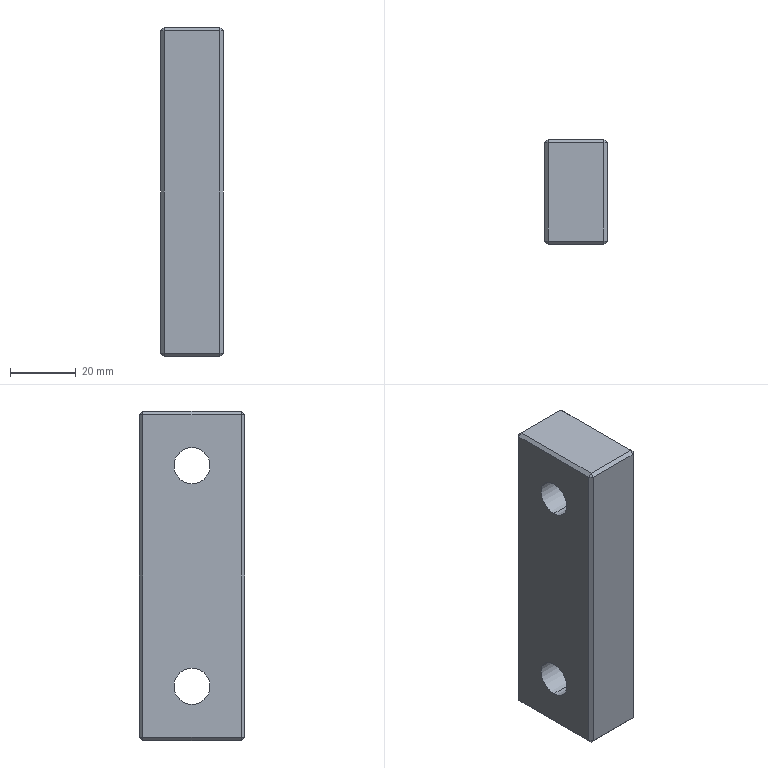Part | SolidWorks | features BaseBody 1 | 1 solid | 36 faces | box 19 x 32 x 100 mm | volume 53384 mm3 | plane 28 | cylinder 8 | commonest cylinder face diameters 11 x4 18 x4
STEP:
#1=CARTESIAN_POINT('',(444.,255.,-24.5));
#2=VERTEX_POINT('',#1);
#3=CARTESIAN_POINT('',(444.,255.,-42.5));
#4=VERTEX_POINT('',#3);
#5=CARTESIAN_POINT('',(444.,255.,-33.5));
#6=DIRECTION('',(1.,0.,0.));
#7=DIRECTION('',(0.,0.,1.));
#8=AXIS2_PLACEMENT_3D('',#5,#6,#7);
#9=CIRCLE('',#8,9.);
#10=EDGE_CURVE('',#2,#4,#9,.T.);
#11=ORIENTED_EDGE('',*,*,#10,.T.);
#12=CARTESIAN_POINT('',(433.,255.,-42.5));
#13=VERTEX_POINT('',#12);
#14=CARTESIAN_POINT('',(444.,255.,-42.5));
#15=DIRECTION('',(-1.,0.,0.));
#16=VECTOR('',#15,1000.);
#17=LINE('',#14,#16);
#18=EDGE_CURVE('',#4,#13,#17,.T.);
#19=ORIENTED_EDGE('',*,*,#18,.T.);
#20=CARTESIAN_POINT('',(433.,255.,-24.5));
#21=VERTEX_POINT('',#20);
#22=CARTESIAN_POINT('',(433.,255.,-33.5));
#23=DIRECTION('',(1.,0.,0.));
#24=DIRECTION('',(0.,0.,1.));
#25=AXIS2_PLACEMENT_3D('',#22,#23,#24);
#26=CIRCLE('',#25,9.);
#27=EDGE_CURVE('',#21,#13,#26,.T.);
#28=ORIENTED_EDGE('',*,*,#27,.F.);
#29=CARTESIAN_POINT('',(444.,255.,-24.5));
#30=DIRECTION('',(-1.,0.,0.));
#31=VECTOR('',#30,1000.);
#32=LINE('',#29,#31);
#33=EDGE_CURVE('',#2,#21,#32,.T.);
#34=ORIENTED_EDGE('',*,*,#33,.F.);
#35=EDGE_LOOP('',(#11,#19,#28,#34));
#36=FACE_OUTER_BOUND('',#35,.T.);
#37=CARTESIAN_POINT('',(444.,255.,-33.5));
#38=DIRECTION('',(-1.,0.,0.));
#39=DIRECTION('',(0.,0.,1.));
#40=AXIS2_PLACEMENT_3D('',#37,#38,#39);
#41=CYLINDRICAL_SURFACE('',#40,9.);
#42=ADVANCED_FACE('',(#36),#41,.F.);
#43=CARTESIAN_POINT('',(433.,255.,-39.));
#44=VERTEX_POINT('',#43);
#45=CARTESIAN_POINT('',(433.,255.,-28.));
#46=VERTEX_POINT('',#45);
#47=CARTESIAN_POINT('',(433.,255.,-33.5));
#48=DIRECTION('',(1.,0.,0.));
#49=DIRECTION('',(0.,0.,1.));
#50=AXIS2_PLACEMENT_3D('',#47,#48,#49);
#51=CIRCLE('',#50,5.5);
#52=EDGE_CURVE('',#44,#46,#51,.T.);
#53=ORIENTED_EDGE('',*,*,#52,.T.);
#54=CARTESIAN_POINT('',(425.,255.,-28.));
#55=VERTEX_POINT('',#54);
#56=CARTESIAN_POINT('',(-56.,255.,-28.));
#57=DIRECTION('',(-1.,0.,0.));
#58=VECTOR('',#57,1000.);
#59=LINE('',#56,#58);
#60=EDGE_CURVE('',#46,#55,#59,.T.);
#61=ORIENTED_EDGE('',*,*,#60,.T.);
#62=CARTESIAN_POINT('',(425.,255.,-39.));
#63=VERTEX_POINT('',#62);
#64=CARTESIAN_POINT('',(425.,255.,-33.5));
#65=DIRECTION('',(1.,0.,0.));
#66=DIRECTION('',(0.,0.,1.));
#67=AXIS2_PLACEMENT_3D('',#64,#65,#66);
#68=CIRCLE('',#67,5.5);
#69=EDGE_CURVE('',#63,#55,#68,.T.);
#70=ORIENTED_EDGE('',*,*,#69,.F.);
#71=CARTESIAN_POINT('',(-56.,255.,-39.));
#72=DIRECTION('',(-1.,0.,0.));
#73=VECTOR('',#72,1000.);
#74=LINE('',#71,#73);
#75=EDGE_CURVE('',#44,#63,#74,.T.);
#76=ORIENTED_EDGE('',*,*,#75,.F.);
#77=EDGE_LOOP('',(#53,#61,#70,#76));
#78=FACE_OUTER_BOUND('',#77,.T.);
#79=CARTESIAN_POINT('',(-56.,255.,-33.5));
#80=DIRECTION('',(-1.,0.,0.));
#81=DIRECTION('',(0.,0.,-1.));
#82=AXIS2_PLACEMENT_3D('',#79,#80,#81);
#83=CYLINDRICAL_SURFACE('',#82,5.5);
#84=ADVANCED_FACE('',(#78),#83,.F.);
#85=CARTESIAN_POINT('',(444.,255.,42.5));
#86=VERTEX_POINT('',#85);
#87=CARTESIAN_POINT('',(444.,255.,24.5));
#88=VERTEX_POINT('',#87);
#89=CARTESIAN_POINT('',(444.,255.,33.5));
#90=DIRECTION('',(1.,0.,0.));
#91=DIRECTION('',(0.,0.,1.));
#92=AXIS2_PLACEMENT_3D('',#89,#90,#91);
#93=CIRCLE('',#92,9.);
#94=EDGE_CURVE('',#86,#88,#93,.T.);
#95=ORIENTED_EDGE('',*,*,#94,.T.);
#96=CARTESIAN_POINT('',(433.,255.,24.5));
#97=VERTEX_POINT('',#96);
#98=CARTESIAN_POINT('',(444.,255.,24.5));
#99=DIRECTION('',(-1.,0.,0.));
#100=VECTOR('',#99,1000.);
#101=LINE('',#98,#100);
#102=EDGE_CURVE('',#88,#97,#101,.T.);
#103=ORIENTED_EDGE('',*,*,#102,.T.);
#104=CARTESIAN_POINT('',(433.,255.,42.5));
#105=VERTEX_POINT('',#104);
#106=CARTESIAN_POINT('',(433.,255.,33.5));
#107=DIRECTION('',(1.,0.,0.));
#108=DIRECTION('',(0.,0.,1.));
#109=AXIS2_PLACEMENT_3D('',#106,#107,#108);
#110=CIRCLE('',#109,9.);
#111=EDGE_CURVE('',#105,#97,#110,.T.);
#112=ORIENTED_EDGE('',*,*,#111,.F.);
#113=CARTESIAN_POINT('',(444.,255.,42.5));
#114=DIRECTION('',(-1.,0.,0.));
#115=VECTOR('',#114,1000.);
#116=LINE('',#113,#115);
#117=EDGE_CURVE('',#86,#105,#116,.T.);
#118=ORIENTED_EDGE('',*,*,#117,.F.);
#119=EDGE_LOOP('',(#95,#103,#112,#118));
#120=FACE_OUTER_BOUND('',#119,.T.);
#121=CARTESIAN_POINT('',(444.,255.,33.5));
#122=DIRECTION('',(-1.,0.,0.));
#123=DIRECTION('',(0.,0.,1.));
#124=AXIS2_PLACEMENT_3D('',#121,#122,#123);
#125=CYLINDRICAL_SURFACE('',#124,9.);
#126=ADVANCED_FACE('',(#120),#125,.F.);
#127=CARTESIAN_POINT('',(433.,255.,28.));
#128=VERTEX_POINT('',#127);
#129=CARTESIAN_POINT('',(433.,255.,39.));
#130=VERTEX_POINT('',#129);
#131=CARTESIAN_POINT('',(433.,255.,33.5));
#132=DIRECTION('',(1.,0.,0.));
#133=DIRECTION('',(0.,0.,1.));
#134=AXIS2_PLACEMENT_3D('',#131,#132,#133);
#135=CIRCLE('',#134,5.5);
#136=EDGE_CURVE('',#128,#130,#135,.T.);
#137=ORIENTED_EDGE('',*,*,#136,.T.);
#138=CARTESIAN_POINT('',(425.,255.,39.));
#139=VERTEX_POINT('',#138);
#140=CARTESIAN_POINT('',(-56.,255.,39.));
#141=DIRECTION('',(-1.,0.,0.));
#142=VECTOR('',#141,1000.);
#143=LINE('',#140,#142);
#144=EDGE_CURVE('',#130,#139,#143,.T.);
#145=ORIENTED_EDGE('',*,*,#144,.T.);
#146=CARTESIAN_POINT('',(425.,255.,28.));
#147=VERTEX_POINT('',#146);
#148=CARTESIAN_POINT('',(425.,255.,33.5));
#149=DIRECTION('',(1.,0.,0.));
#150=DIRECTION('',(0.,0.,1.));
#151=AXIS2_PLACEMENT_3D('',#148,#149,#150);
#152=CIRCLE('',#151,5.5);
#153=EDGE_CURVE('',#147,#139,#152,.T.);
#154=ORIENTED_EDGE('',*,*,#153,.F.);
#155=CARTESIAN_POINT('',(-56.,255.,28.));
#156=DIRECTION('',(-1.,0.,0.));
#157=VECTOR('',#156,1000.);
#158=LINE('',#155,#157);
#159=EDGE_CURVE('',#128,#147,#158,.T.);
#160=ORIENTED_EDGE('',*,*,#159,.F.);
#161=EDGE_LOOP('',(#137,#145,#154,#160));
#162=FACE_OUTER_BOUND('',#161,.T.);
#163=CARTESIAN_POINT('',(-56.,255.,33.5));
#164=DIRECTION('',(-1.,0.,0.));
#165=DIRECTION('',(0.,0.,-1.));
#166=AXIS2_PLACEMENT_3D('',#163,#164,#165);
#167=CYLINDRICAL_SURFACE('',#166,5.5);
#168=ADVANCED_FACE('',(#162),#167,.F.);
#169=CARTESIAN_POINT('',(426.,271.,49.));
#170=VERTEX_POINT('',#169);
#171=CARTESIAN_POINT('',(426.,271.,-49.));
#172=VERTEX_POINT('',#171);
#173=CARTESIAN_POINT('',(426.,271.,-60.));
#174=DIRECTION('',(0.,0.,-1.));
#175=VECTOR('',#174,1000.);
#176=LINE('',#173,#175);
#177=EDGE_CURVE('',#170,#172,#176,.T.);
#178=ORIENTED_EDGE('',*,*,#177,.F.);
#179=CARTESIAN_POINT('',(443.,271.,49.));
#180=VERTEX_POINT('',#179);
#181=CARTESIAN_POINT('',(434.5,271.,49.));
#182=DIRECTION('',(-1.,0.,0.));
#183=VECTOR('',#182,1000.);
#184=LINE('',#181,#183);
#185=EDGE_CURVE('',#180,#170,#184,.T.);
#186=ORIENTED_EDGE('',*,*,#185,.F.);
#187=CARTESIAN_POINT('',(443.,271.,-49.));
#188=VERTEX_POINT('',#187);
#189=CARTESIAN_POINT('',(443.,271.,-60.));
#190=DIRECTION('',(0.,0.,1.));
#191=VECTOR('',#190,1000.);
#192=LINE('',#189,#191);
#193=EDGE_CURVE('',#188,#180,#192,.T.);
#194=ORIENTED_EDGE('',*,*,#193,.F.);
#195=CARTESIAN_POINT('',(444.,271.,-49.));
#196=DIRECTION('',(1.,0.,0.));
#197=VECTOR('',#196,1000.);
#198=LINE('',#195,#197);
#199=EDGE_CURVE('',#172,#188,#198,.T.);
#200=ORIENTED_EDGE('',*,*,#199,.F.);
#201=EDGE_LOOP('',(#178,#186,#194,#200));
#202=FACE_OUTER_BOUND('',#201,.T.);
#203=CARTESIAN_POINT('',(434.5,271.,-60.));
#204=DIRECTION('',(0.,1.,0.));
#205=DIRECTION('',(0.,0.,-1.));
#206=AXIS2_PLACEMENT_3D('',#203,#204,#205);
#207=PLANE('',#206);
#208=ADVANCED_FACE('',(#202),#207,.T.);
#209=CARTESIAN_POINT('',(426.,270.,-50.));
#210=VERTEX_POINT('',#209);
#211=CARTESIAN_POINT('',(426.,240.,-50.));
#212=VERTEX_POINT('',#211);
#213=CARTESIAN_POINT('',(426.,239.,-50.));
#214=DIRECTION('',(0.,-1.,0.));
#215=VECTOR('',#214,1000.);
#216=LINE('',#213,#215);
#217=EDGE_CURVE('',#210,#212,#216,.T.);
#218=ORIENTED_EDGE('',*,*,#217,.F.);
#219=CARTESIAN_POINT('',(443.,270.,-50.));
#220=VERTEX_POINT('',#219);
#221=CARTESIAN_POINT('',(425.,270.,-50.));
#222=DIRECTION('',(-1.,0.,0.));
#223=VECTOR('',#222,1000.);
#224=LINE('',#221,#223);
#225=EDGE_CURVE('',#220,#210,#224,.T.);
#226=ORIENTED_EDGE('',*,*,#225,.F.);
#227=CARTESIAN_POINT('',(443.,240.,-50.));
#228=VERTEX_POINT('',#227);
#229=CARTESIAN_POINT('',(443.,271.,-50.));
#230=DIRECTION('',(0.,1.,0.));
#231=VECTOR('',#230,1000.);
#232=LINE('',#229,#231);
#233=EDGE_CURVE('',#228,#220,#232,.T.);
#234=ORIENTED_EDGE('',*,*,#233,.F.);
#235=CARTESIAN_POINT('',(135.,240.,-50.));
#236=DIRECTION('',(1.,0.,0.));
#237=VECTOR('',#236,1000.);
#238=LINE('',#235,#237);
#239=EDGE_CURVE('',#212,#228,#238,.T.);
#240=ORIENTED_EDGE('',*,*,#239,.F.);
#241=EDGE_LOOP('',(#218,#226,#234,#240));
#242=FACE_OUTER_BOUND('',#241,.T.);
#243=CARTESIAN_POINT('',(135.,111.,-50.));
#244=DIRECTION('',(0.,0.,1.));
#245=DIRECTION('',(1.,0.,0.));
#246=AXIS2_PLACEMENT_3D('',#243,#244,#245);
#247=PLANE('',#246);
#248=ADVANCED_FACE('',(#242),#247,.F.);
#249=ORIENTED_EDGE('',*,*,#10,.F.);
#250=CARTESIAN_POINT('',(444.,255.,-33.5));
#251=DIRECTION('',(1.,0.,0.));
#252=DIRECTION('',(0.,0.,1.));
#253=AXIS2_PLACEMENT_3D('',#250,#251,#252);
#254=CIRCLE('',#253,9.);
#255=EDGE_CURVE('',#4,#2,#254,.T.);
#256=ORIENTED_EDGE('',*,*,#255,.F.);
#257=EDGE_LOOP('',(#249,#256));
#258=FACE_BOUND('',#257,.T.);
#259=ORIENTED_EDGE('',*,*,#94,.F.);
#260=CARTESIAN_POINT('',(444.,255.,33.5));
#261=DIRECTION('',(1.,0.,0.));
#262=DIRECTION('',(0.,0.,1.));
#263=AXIS2_PLACEMENT_3D('',#260,#261,#262);
#264=CIRCLE('',#263,9.);
#265=EDGE_CURVE('',#88,#86,#264,.T.);
#266=ORIENTED_EDGE('',*,*,#265,.F.);
#267=EDGE_LOOP('',(#259,#266));
#268=FACE_BOUND('',#267,.T.);
#269=CARTESIAN_POINT('',(444.,270.,49.));
#270=VERTEX_POINT('',#269);
#271=CARTESIAN_POINT('',(444.,270.,-49.));
#272=VERTEX_POINT('',#271);
#273=CARTESIAN_POINT('',(444.,270.,-60.));
#274=DIRECTION('',(0.,0.,-1.));
#275=VECTOR('',#274,1000.);
#276=LINE('',#273,#275);
#277=EDGE_CURVE('',#270,#272,#276,.T.);
#278=ORIENTED_EDGE('',*,*,#277,.F.);
#279=CARTESIAN_POINT('',(444.,240.,49.));
#280=VERTEX_POINT('',#279);
#281=CARTESIAN_POINT('',(444.,251.,49.));
#282=DIRECTION('',(0.,1.,0.));
#283=VECTOR('',#282,1000.);
#284=LINE('',#281,#283);
#285=EDGE_CURVE('',#280,#270,#284,.T.);
#286=ORIENTED_EDGE('',*,*,#285,.F.);
#287=CARTESIAN_POINT('',(444.,240.,-49.));
#288=VERTEX_POINT('',#287);
#289=CARTESIAN_POINT('',(444.,240.,50.));
#290=DIRECTION('',(0.,0.,1.));
#291=VECTOR('',#290,1000.);
#292=LINE('',#289,#291);
#293=EDGE_CURVE('',#288,#280,#292,.T.);
#294=ORIENTED_EDGE('',*,*,#293,.F.);
#295=CARTESIAN_POINT('',(444.,239.,-49.));
#296=DIRECTION('',(0.,-1.,0.));
#297=VECTOR('',#296,1000.);
#298=LINE('',#295,#297);
#299=EDGE_CURVE('',#272,#288,#298,.T.);
#300=ORIENTED_EDGE('',*,*,#299,.F.);
#301=EDGE_LOOP('',(#278,#286,#294,#300));
#302=FACE_OUTER_BOUND('',#301,.T.);
#303=CARTESIAN_POINT('',(444.,251.,-60.));
#304=DIRECTION('',(1.,0.,0.));
#305=DIRECTION('',(0.,0.,-1.));
#306=AXIS2_PLACEMENT_3D('',#303,#304,#305);
#307=PLANE('',#306);
#308=ADVANCED_FACE('',(#258,#268,#302),#307,.T.);
#309=ORIENTED_EDGE('',*,*,#69,.T.);
#310=CARTESIAN_POINT('',(425.,255.,-33.5));
#311=DIRECTION('',(1.,0.,0.));
#312=DIRECTION('',(0.,0.,1.));
#313=AXIS2_PLACEMENT_3D('',#310,#311,#312);
#314=CIRCLE('',#313,5.5);
#315=EDGE_CURVE('',#55,#63,#314,.T.);
#316=ORIENTED_EDGE('',*,*,#315,.T.);
#317=EDGE_LOOP('',(#309,#316));
#318=FACE_BOUND('',#317,.T.);
#319=ORIENTED_EDGE('',*,*,#153,.T.);
#320=CARTESIAN_POINT('',(425.,255.,33.5));
#321=DIRECTION('',(1.,0.,0.));
#322=DIRECTION('',(0.,0.,1.));
#323=AXIS2_PLACEMENT_3D('',#320,#321,#322);
#324=CIRCLE('',#323,5.5);
#325=EDGE_CURVE('',#139,#147,#324,.T.);
#326=ORIENTED_EDGE('',*,*,#325,.T.);
#327=EDGE_LOOP('',(#319,#326));
#328=FACE_BOUND('',#327,.T.);
#329=CARTESIAN_POINT('',(425.,240.,-49.));
#330=VERTEX_POINT('',#329);
#331=CARTESIAN_POINT('',(425.,270.,-49.));
#332=VERTEX_POINT('',#331);
#333=CARTESIAN_POINT('',(425.,271.,-49.));
#334=DIRECTION('',(0.,1.,0.));
#335=VECTOR('',#334,1000.);
#336=LINE('',#333,#335);
#337=EDGE_CURVE('',#330,#332,#336,.T.);
#338=ORIENTED_EDGE('',*,*,#337,.F.);
#339=CARTESIAN_POINT('',(425.,240.,49.));
#340=VERTEX_POINT('',#339);
#341=CARTESIAN_POINT('',(425.,240.,-50.));
#342=DIRECTION('',(0.,0.,-1.));
#343=VECTOR('',#342,1000.);
#344=LINE('',#341,#343);
#345=EDGE_CURVE('',#340,#330,#344,.T.);
#346=ORIENTED_EDGE('',*,*,#345,.F.);
#347=CARTESIAN_POINT('',(425.,270.,49.));
#348=VERTEX_POINT('',#347);
#349=CARTESIAN_POINT('',(425.,251.,49.));
#350=DIRECTION('',(0.,-1.,0.));
#351=VECTOR('',#350,1000.);
#352=LINE('',#349,#351);
#353=EDGE_CURVE('',#348,#340,#352,.T.);
#354=ORIENTED_EDGE('',*,*,#353,.F.);
#355=CARTESIAN_POINT('',(425.,270.,-60.));
#356=DIRECTION('',(0.,0.,1.));
#357=VECTOR('',#356,1000.);
#358=LINE('',#355,#357);
#359=EDGE_CURVE('',#332,#348,#358,.T.);
#360=ORIENTED_EDGE('',*,*,#359,.F.);
#361=EDGE_LOOP('',(#338,#346,#354,#360));
#362=FACE_OUTER_BOUND('',#361,.T.);
#363=CARTESIAN_POINT('',(425.,251.,-60.));
#364=DIRECTION('',(-1.,0.,0.));
#365=DIRECTION('',(0.,0.,1.));
#366=AXIS2_PLACEMENT_3D('',#363,#364,#365);
#367=PLANE('',#366);
#368=ADVANCED_FACE('',(#318,#328,#362),#367,.T.);
#369=CARTESIAN_POINT('',(443.,270.,50.));
#370=VERTEX_POINT('',#369);
#371=CARTESIAN_POINT('',(443.,240.,50.));
#372=VERTEX_POINT('',#371);
#373=CARTESIAN_POINT('',(443.,251.,50.));
#374=DIRECTION('',(0.,-1.,0.));
#375=VECTOR('',#374,1000.);
#376=LINE('',#373,#375);
#377=EDGE_CURVE('',#370,#372,#376,.T.);
#378=ORIENTED_EDGE('',*,*,#377,.F.);
#379=CARTESIAN_POINT('',(426.,270.,50.));
#380=VERTEX_POINT('',#379);
#381=CARTESIAN_POINT('',(434.5,270.,50.));
#382=DIRECTION('',(1.,0.,0.));
#383=VECTOR('',#382,1000.);
#384=LINE('',#381,#383);
#385=EDGE_CURVE('',#380,#370,#384,.T.);
#386=ORIENTED_EDGE('',*,*,#385,.F.);
#387=CARTESIAN_POINT('',(426.,240.,50.));
#388=VERTEX_POINT('',#387);
#389=CARTESIAN_POINT('',(426.,251.,50.));
#390=DIRECTION('',(0.,1.,0.));
#391=VECTOR('',#390,1000.);
#392=LINE('',#389,#391);
#393=EDGE_CURVE('',#388,#380,#392,.T.);
#394=ORIENTED_EDGE('',*,*,#393,.F.);
#395=CARTESIAN_POINT('',(425.,240.,50.));
#396=DIRECTION('',(-1.,0.,0.));
#397=VECTOR('',#396,1000.);
#398=LINE('',#395,#397);
#399=EDGE_CURVE('',#372,#388,#398,.T.);
#400=ORIENTED_EDGE('',*,*,#399,.F.);
#401=EDGE_LOOP('',(#378,#386,#394,#400));
#402=FACE_OUTER_BOUND('',#401,.T.);
#403=CARTESIAN_POINT('',(434.5,251.,50.));
#404=DIRECTION('',(0.,0.,1.));
#405=DIRECTION('',(1.,0.,0.));
#406=AXIS2_PLACEMENT_3D('',#403,#404,#405);
#407=PLANE('',#406);
#408=ADVANCED_FACE('',(#402),#407,.T.);
#409=CARTESIAN_POINT('',(443.,239.,49.));
#410=VERTEX_POINT('',#409);
#411=CARTESIAN_POINT('',(443.,239.,-49.));
#412=VERTEX_POINT('',#411);
#413=CARTESIAN_POINT('',(443.,239.,-50.));
#414=DIRECTION('',(0.,0.,-1.));
#415=VECTOR('',#414,1000.);
#416=LINE('',#413,#415);
#417=EDGE_CURVE('',#410,#412,#416,.T.);
#418=ORIENTED_EDGE('',*,*,#417,.F.);
#419=CARTESIAN_POINT('',(426.,239.,49.));
#420=VERTEX_POINT('',#419);
#421=CARTESIAN_POINT('',(444.,239.,49.));
#422=DIRECTION('',(1.,0.,0.));
#423=VECTOR('',#422,1000.);
#424=LINE('',#421,#423);
#425=EDGE_CURVE('',#420,#410,#424,.T.);
#426=ORIENTED_EDGE('',*,*,#425,.F.);
#427=CARTESIAN_POINT('',(426.,239.,-49.));
#428=VERTEX_POINT('',#427);
#429=CARTESIAN_POINT('',(426.,239.,50.));
#430=DIRECTION('',(0.,0.,1.));
#431=VECTOR('',#430,1000.);
#432=LINE('',#429,#431);
#433=EDGE_CURVE('',#428,#420,#432,.T.);
#434=ORIENTED_EDGE('',*,*,#433,.F.);
#435=CARTESIAN_POINT('',(434.5,239.,-49.));
#436=DIRECTION('',(-1.,0.,0.));
#437=VECTOR('',#436,1000.);
#438=LINE('',#435,#437);
#439=EDGE_CURVE('',#412,#428,#438,.T.);
#440=ORIENTED_EDGE('',*,*,#439,.F.);
#441=EDGE_LOOP('',(#418,#426,#434,#440));
#442=FACE_OUTER_BOUND('',#441,.T.);
#443=CARTESIAN_POINT('',(434.5,239.,0.));
#444=DIRECTION('',(0.,1.,0.));
#445=DIRECTION('',(0.,0.,-1.));
#446=AXIS2_PLACEMENT_3D('',#443,#444,#445);
#447=PLANE('',#446);
#448=ADVANCED_FACE('',(#442),#447,.F.);
#449=CARTESIAN_POINT('',(426.,270.5,49.5));
#450=DIRECTION('',(0.,-0.7071,0.7071));
#451=VECTOR('',#450,1000.);
#452=LINE('',#449,#451);
#453=EDGE_CURVE('',#170,#380,#452,.T.);
#454=ORIENTED_EDGE('',*,*,#453,.T.);
#455=ORIENTED_EDGE('',*,*,#385,.T.);
#456=CARTESIAN_POINT('',(443.,271.,49.));
#457=DIRECTION('',(0.,0.7071,-0.7071));
#458=VECTOR('',#457,1000.);
#459=LINE('',#456,#458);
#460=EDGE_CURVE('',#370,#180,#459,.T.);
#461=ORIENTED_EDGE('',*,*,#460,.T.);
#462=ORIENTED_EDGE('',*,*,#185,.T.);
#463=EDGE_LOOP('',(#454,#455,#461,#462));
#464=FACE_OUTER_BOUND('',#463,.T.);
#465=CARTESIAN_POINT('',(434.5,271.,49.));
#466=DIRECTION('',(0.,-0.7071,-0.7071));
#467=DIRECTION('',(0.,-0.7071,0.7071));
#468=AXIS2_PLACEMENT_3D('',#465,#466,#467);
#469=PLANE('',#468);
#470=ADVANCED_FACE('',(#464),#469,.F.);
#471=CARTESIAN_POINT('',(425.,270.,49.));
#472=DIRECTION('',(-0.7071,-0.7071,0.));
#473=VECTOR('',#472,1000.);
#474=LINE('',#471,#473);
#475=EDGE_CURVE('',#170,#348,#474,.T.);
#476=ORIENTED_EDGE('',*,*,#475,.T.);
#477=CARTESIAN_POINT('',(425.,270.,49.));
#478=DIRECTION('',(0.7071,0.,0.7071));
#479=VECTOR('',#478,1000.);
#480=LINE('',#477,#479);
#481=EDGE_CURVE('',#348,#380,#480,.T.);
#482=ORIENTED_EDGE('',*,*,#481,.T.);
#483=ORIENTED_EDGE('',*,*,#453,.F.);
#484=EDGE_LOOP('',(#476,#482,#483));
#485=FACE_OUTER_BOUND('',#484,.T.);
#486=CARTESIAN_POINT('',(425.,270.,49.));
#487=DIRECTION('',(-0.5774,0.5774,0.5774));
#488=DIRECTION('',(0.7071,0.,0.7071));
#489=AXIS2_PLACEMENT_3D('',#486,#487,#488);
#490=PLANE('',#489);
#491=ADVANCED_FACE('',(#485),#490,.T.);
#492=CARTESIAN_POINT('',(443.5,270.,49.5));
#493=DIRECTION('',(0.7071,0.,-0.7071));
#494=VECTOR('',#493,1000.);
#495=LINE('',#492,#494);
#496=EDGE_CURVE('',#370,#270,#495,.T.);
#497=ORIENTED_EDGE('',*,*,#496,.T.);
#498=CARTESIAN_POINT('',(443.,271.,49.));
#499=DIRECTION('',(-0.7071,0.7071,0.));
#500=VECTOR('',#499,1000.);
#501=LINE('',#498,#500);
#502=EDGE_CURVE('',#270,#180,#501,.T.);
#503=ORIENTED_EDGE('',*,*,#502,.T.);
#504=ORIENTED_EDGE('',*,*,#460,.F.);
#505=EDGE_LOOP('',(#497,#503,#504));
#506=FACE_OUTER_BOUND('',#505,.T.);
#507=CARTESIAN_POINT('',(443.,271.,49.));
#508=DIRECTION('',(0.5774,0.5774,0.5774));
#509=DIRECTION('',(0.7071,0.,-0.7071));
#510=AXIS2_PLACEMENT_3D('',#507,#508,#509);
#511=PLANE('',#510);
#512=ADVANCED_FACE('',(#506),#511,.T.);
#513=ORIENTED_EDGE('',*,*,#481,.F.);
#514=ORIENTED_EDGE('',*,*,#353,.T.);
#515=CARTESIAN_POINT('',(426.,240.,50.));
#516=DIRECTION('',(0.7071,0.,0.7071));
#517=VECTOR('',#516,1000.);
#518=LINE('',#515,#517);
#519=EDGE_CURVE('',#340,#388,#518,.T.);
#520=ORIENTED_EDGE('',*,*,#519,.T.);
#521=ORIENTED_EDGE('',*,*,#393,.T.);
#522=EDGE_LOOP('',(#513,#514,#520,#521));
#523=FACE_OUTER_BOUND('',#522,.T.);
#524=CARTESIAN_POINT('',(425.,251.,49.));
#525=DIRECTION('',(0.7071,0.,-0.7071));
#526=DIRECTION('',(-0.7071,0.,-0.7071));
#527=AXIS2_PLACEMENT_3D('',#524,#525,#526);
#528=PLANE('',#527);
#529=ADVANCED_FACE('',(#523),#528,.F.);
#530=ORIENTED_EDGE('',*,*,#475,.F.);
#531=ORIENTED_EDGE('',*,*,#177,.T.);
#532=CARTESIAN_POINT('',(426.,271.,-49.));
#533=DIRECTION('',(-0.7071,-0.7071,0.));
#534=VECTOR('',#533,1000.);
#535=LINE('',#532,#534);
#536=EDGE_CURVE('',#172,#332,#535,.T.);
#537=ORIENTED_EDGE('',*,*,#536,.T.);
#538=ORIENTED_EDGE('',*,*,#359,.T.);
#539=EDGE_LOOP('',(#530,#531,#537,#538));
#540=FACE_OUTER_BOUND('',#539,.T.);
#541=CARTESIAN_POINT('',(425.,270.,-60.));
#542=DIRECTION('',(0.7071,-0.7071,0.));
#543=DIRECTION('',(-0.7071,-0.7071,0.));
#544=AXIS2_PLACEMENT_3D('',#541,#542,#543);
#545=PLANE('',#544);
#546=ADVANCED_FACE('',(#540),#545,.F.);
#547=CARTESIAN_POINT('',(443.,270.,-50.));
#548=DIRECTION('',(0.,-0.7071,-0.7071));
#549=VECTOR('',#548,1000.);
#550=LINE('',#547,#549);
#551=EDGE_CURVE('',#188,#220,#550,.T.);
#552=ORIENTED_EDGE('',*,*,#551,.T.);
#553=ORIENTED_EDGE('',*,*,#225,.T.);
#554=CARTESIAN_POINT('',(426.,271.,-49.));
#555=DIRECTION('',(0.,0.7071,0.7071));
#556=VECTOR('',#555,1000.);
#557=LINE('',#554,#556);
#558=EDGE_CURVE('',#210,#172,#557,.T.);
#559=ORIENTED_EDGE('',*,*,#558,.T.);
#560=ORIENTED_EDGE('',*,*,#199,.T.);
#561=EDGE_LOOP('',(#552,#553,#559,#560));
#562=FACE_OUTER_BOUND('',#561,.T.);
#563=CARTESIAN_POINT('',(135.,270.,-50.));
#564=DIRECTION('',(0.,0.7071,-0.7071));
#565=DIRECTION('',(0.,-0.7071,-0.7071));
#566=AXIS2_PLACEMENT_3D('',#563,#564,#565);
#567=PLANE('',#566);
#568=ADVANCED_FACE('',(#562),#567,.T.);
#569=ORIENTED_EDGE('',*,*,#502,.F.);
#570=ORIENTED_EDGE('',*,*,#277,.T.);
#571=CARTESIAN_POINT('',(443.5,270.5,-49.));
#572=DIRECTION('',(-0.7071,0.7071,0.));
#573=VECTOR('',#572,1000.);
#574=LINE('',#571,#573);
#575=EDGE_CURVE('',#272,#188,#574,.T.);
#576=ORIENTED_EDGE('',*,*,#575,.T.);
#577=ORIENTED_EDGE('',*,*,#193,.T.);
#578=EDGE_LOOP('',(#569,#570,#576,#577));
#579=FACE_OUTER_BOUND('',#578,.T.);
#580=CARTESIAN_POINT('',(443.,271.,-60.));
#581=DIRECTION('',(-0.7071,-0.7071,0.));
#582=DIRECTION('',(-0.7071,0.7071,0.));
#583=AXIS2_PLACEMENT_3D('',#580,#581,#582);
#584=PLANE('',#583);
#585=ADVANCED_FACE('',(#579),#584,.F.);
#586=ORIENTED_EDGE('',*,*,#496,.F.);
#587=ORIENTED_EDGE('',*,*,#377,.T.);
#588=CARTESIAN_POINT('',(444.,240.,49.));
#589=DIRECTION('',(0.7071,0.,-0.7071));
#590=VECTOR('',#589,1000.);
#591=LINE('',#588,#590);
#592=EDGE_CURVE('',#372,#280,#591,.T.);
#593=ORIENTED_EDGE('',*,*,#592,.T.);
#594=ORIENTED_EDGE('',*,*,#285,.T.);
#595=EDGE_LOOP('',(#586,#587,#593,#594));
#596=FACE_OUTER_BOUND('',#595,.T.);
#597=CARTESIAN_POINT('',(444.,251.,49.));
#598=DIRECTION('',(-0.7071,0.,-0.7071));
#599=DIRECTION('',(-0.7071,0.,0.7071));
#600=AXIS2_PLACEMENT_3D('',#597,#598,#599);
#601=PLANE('',#600);
#602=ADVANCED_FACE('',(#596),#601,.F.);
#603=CARTESIAN_POINT('',(426.,240.,50.));
#604=DIRECTION('',(0.,-0.7071,-0.7071));
#605=VECTOR('',#604,1000.);
#606=LINE('',#603,#605);
#607=EDGE_CURVE('',#388,#420,#606,.T.);
#608=ORIENTED_EDGE('',*,*,#607,.T.);
#609=ORIENTED_EDGE('',*,*,#425,.T.);
#610=CARTESIAN_POINT('',(443.,239.5,49.5));
#611=DIRECTION('',(0.,0.7071,0.7071));
#612=VECTOR('',#611,1000.);
#613=LINE('',#610,#612);
#614=EDGE_CURVE('',#410,#372,#613,.T.);
#615=ORIENTED_EDGE('',*,*,#614,.T.);
#616=ORIENTED_EDGE('',*,*,#399,.T.);
#617=EDGE_LOOP('',(#608,#609,#615,#616));
#618=FACE_OUTER_BOUND('',#617,.T.);
#619=CARTESIAN_POINT('',(434.5,239.,49.));
#620=DIRECTION('',(0.,-0.7071,0.7071));
#621=DIRECTION('',(0.,0.7071,0.7071));
#622=AXIS2_PLACEMENT_3D('',#619,#620,#621);
#623=PLANE('',#622);
#624=ADVANCED_FACE('',(#618),#623,.T.);
#625=ORIENTED_EDGE('',*,*,#519,.F.);
#626=CARTESIAN_POINT('',(425.5,239.5,49.));
#627=DIRECTION('',(0.7071,-0.7071,0.));
#628=VECTOR('',#627,1000.);
#629=LINE('',#626,#628);
#630=EDGE_CURVE('',#340,#420,#629,.T.);
#631=ORIENTED_EDGE('',*,*,#630,.T.);
#632=ORIENTED_EDGE('',*,*,#607,.F.);
#633=EDGE_LOOP('',(#625,#631,#632));
#634=FACE_OUTER_BOUND('',#633,.T.);
#635=CARTESIAN_POINT('',(426.,240.,50.));
#636=DIRECTION('',(-0.5774,-0.5774,0.5774));
#637=DIRECTION('',(0.7071,0.,0.7071));
#638=AXIS2_PLACEMENT_3D('',#635,#636,#637);
#639=PLANE('',#638);
#640=ADVANCED_FACE('',(#634),#639,.T.);
#641=ORIENTED_EDGE('',*,*,#558,.F.);
#642=CARTESIAN_POINT('',(425.5,270.,-49.5));
#643=DIRECTION('',(-0.7071,0.,0.7071));
#644=VECTOR('',#643,1000.);
#645=LINE('',#642,#644);
#646=EDGE_CURVE('',#210,#332,#645,.T.);
#647=ORIENTED_EDGE('',*,*,#646,.T.);
#648=ORIENTED_EDGE('',*,*,#536,.F.);
#649=EDGE_LOOP('',(#641,#647,#648));
#650=FACE_OUTER_BOUND('',#649,.T.);
#651=CARTESIAN_POINT('',(426.,271.,-49.));
#652=DIRECTION('',(-0.5774,0.5774,-0.5774));
#653=DIRECTION('',(-0.7071,0.,0.7071));
#654=AXIS2_PLACEMENT_3D('',#651,#652,#653);
#655=PLANE('',#654);
#656=ADVANCED_FACE('',(#650),#655,.T.);
#657=ORIENTED_EDGE('',*,*,#575,.F.);
#658=CARTESIAN_POINT('',(443.,270.,-50.));
#659=DIRECTION('',(-0.7071,0.,-0.7071));
#660=VECTOR('',#659,1000.);
#661=LINE('',#658,#660);
#662=EDGE_CURVE('',#272,#220,#661,.T.);
#663=ORIENTED_EDGE('',*,*,#662,.T.);
#664=ORIENTED_EDGE('',*,*,#551,.F.);
#665=EDGE_LOOP('',(#657,#663,#664));
#666=FACE_OUTER_BOUND('',#665,.T.);
#667=CARTESIAN_POINT('',(443.,270.,-50.));
#668=DIRECTION('',(0.5774,0.5774,-0.5774));
#669=DIRECTION('',(-0.7071,0.,-0.7071));
#670=AXIS2_PLACEMENT_3D('',#667,#668,#669);
#671=PLANE('',#670);
#672=ADVANCED_FACE('',(#666),#671,.T.);
#673=ORIENTED_EDGE('',*,*,#614,.F.);
#674=CARTESIAN_POINT('',(444.,240.,49.));
#675=DIRECTION('',(0.7071,0.7071,0.));
#676=VECTOR('',#675,1000.);
#677=LINE('',#674,#676);
#678=EDGE_CURVE('',#410,#280,#677,.T.);
#679=ORIENTED_EDGE('',*,*,#678,.T.);
#680=ORIENTED_EDGE('',*,*,#592,.F.);
#681=EDGE_LOOP('',(#673,#679,#680));
#682=FACE_OUTER_BOUND('',#681,.T.);
#683=CARTESIAN_POINT('',(444.,240.,49.));
#684=DIRECTION('',(0.5774,-0.5774,0.5774));
#685=DIRECTION('',(0.7071,0.,-0.7071));
#686=AXIS2_PLACEMENT_3D('',#683,#684,#685);
#687=PLANE('',#686);
#688=ADVANCED_FACE('',(#682),#687,.T.);
#689=ORIENTED_EDGE('',*,*,#630,.F.);
#690=ORIENTED_EDGE('',*,*,#345,.T.);
#691=CARTESIAN_POINT('',(426.,239.,-49.));
#692=DIRECTION('',(0.7071,-0.7071,0.));
#693=VECTOR('',#692,1000.);
#694=LINE('',#691,#693);
#695=EDGE_CURVE('',#330,#428,#694,.T.);
#696=ORIENTED_EDGE('',*,*,#695,.T.);
#697=ORIENTED_EDGE('',*,*,#433,.T.);
#698=EDGE_LOOP('',(#689,#690,#696,#697));
#699=FACE_OUTER_BOUND('',#698,.T.);
#700=CARTESIAN_POINT('',(426.,239.,0.));
#701=DIRECTION('',(-0.7071,-0.7071,0.));
#702=DIRECTION('',(-0.7071,0.7071,0.));
#703=AXIS2_PLACEMENT_3D('',#700,#701,#702);
#704=PLANE('',#703);
#705=ADVANCED_FACE('',(#699),#704,.T.);
#706=ORIENTED_EDGE('',*,*,#646,.F.);
#707=ORIENTED_EDGE('',*,*,#217,.T.);
#708=CARTESIAN_POINT('',(425.5,240.,-49.5));
#709=DIRECTION('',(-0.7071,0.,0.7071));
#710=VECTOR('',#709,1000.);
#711=LINE('',#708,#710);
#712=EDGE_CURVE('',#212,#330,#711,.T.);
#713=ORIENTED_EDGE('',*,*,#712,.T.);
#714=ORIENTED_EDGE('',*,*,#337,.T.);
#715=EDGE_LOOP('',(#706,#707,#713,#714));
#716=FACE_OUTER_BOUND('',#715,.T.);
#717=CARTESIAN_POINT('',(426.,111.,-50.));
#718=DIRECTION('',(-0.7071,0.,-0.7071));
#719=DIRECTION('',(-0.7071,0.,0.7071));
#720=AXIS2_PLACEMENT_3D('',#717,#718,#719);
#721=PLANE('',#720);
#722=ADVANCED_FACE('',(#716),#721,.T.);
#723=ORIENTED_EDGE('',*,*,#662,.F.);
#724=ORIENTED_EDGE('',*,*,#299,.T.);
#725=CARTESIAN_POINT('',(443.,240.,-50.));
#726=DIRECTION('',(-0.7071,0.,-0.7071));
#727=VECTOR('',#726,1000.);
#728=LINE('',#725,#727);
#729=EDGE_CURVE('',#288,#228,#728,.T.);
#730=ORIENTED_EDGE('',*,*,#729,.T.);
#731=ORIENTED_EDGE('',*,*,#233,.T.);
#732=EDGE_LOOP('',(#723,#724,#730,#731));
#733=FACE_OUTER_BOUND('',#732,.T.);
#734=CARTESIAN_POINT('',(443.,111.,-50.));
#735=DIRECTION('',(0.7071,0.,-0.7071));
#736=DIRECTION('',(-0.7071,0.,-0.7071));
#737=AXIS2_PLACEMENT_3D('',#734,#735,#736);
#738=PLANE('',#737);
#739=ADVANCED_FACE('',(#733),#738,.T.);
#740=ORIENTED_EDGE('',*,*,#678,.F.);
#741=ORIENTED_EDGE('',*,*,#417,.T.);
#742=CARTESIAN_POINT('',(443.5,239.5,-49.));
#743=DIRECTION('',(0.7071,0.7071,0.));
#744=VECTOR('',#743,1000.);
#745=LINE('',#742,#744);
#746=EDGE_CURVE('',#412,#288,#745,.T.);
#747=ORIENTED_EDGE('',*,*,#746,.T.);
#748=ORIENTED_EDGE('',*,*,#293,.T.);
#749=EDGE_LOOP('',(#740,#741,#747,#748));
#750=FACE_OUTER_BOUND('',#749,.T.);
#751=CARTESIAN_POINT('',(443.,239.,0.));
#752=DIRECTION('',(0.7071,-0.7071,0.));
#753=DIRECTION('',(-0.7071,-0.7071,0.));
#754=AXIS2_PLACEMENT_3D('',#751,#752,#753);
#755=PLANE('',#754);
#756=ADVANCED_FACE('',(#750),#755,.T.);
#757=ORIENTED_EDGE('',*,*,#712,.F.);
#758=CARTESIAN_POINT('',(426.,239.,-49.));
#759=DIRECTION('',(0.,-0.7071,0.7071));
#760=VECTOR('',#759,1000.);
#761=LINE('',#758,#760);
#762=EDGE_CURVE('',#212,#428,#761,.T.);
#763=ORIENTED_EDGE('',*,*,#762,.T.);
#764=ORIENTED_EDGE('',*,*,#695,.F.);
#765=EDGE_LOOP('',(#757,#763,#764));
#766=FACE_OUTER_BOUND('',#765,.T.);
#767=CARTESIAN_POINT('',(426.,239.,-49.));
#768=DIRECTION('',(-0.5774,-0.5774,-0.5774));
#769=DIRECTION('',(-0.7071,0.,0.7071));
#770=AXIS2_PLACEMENT_3D('',#767,#768,#769);
#771=PLANE('',#770);
#772=ADVANCED_FACE('',(#766),#771,.T.);
#773=ORIENTED_EDGE('',*,*,#746,.F.);
#774=CARTESIAN_POINT('',(443.,240.,-50.));
#775=DIRECTION('',(0.,0.7071,-0.7071));
#776=VECTOR('',#775,1000.);
#777=LINE('',#774,#776);
#778=EDGE_CURVE('',#412,#228,#777,.T.);
#779=ORIENTED_EDGE('',*,*,#778,.T.);
#780=ORIENTED_EDGE('',*,*,#729,.F.);
#781=EDGE_LOOP('',(#773,#779,#780));
#782=FACE_OUTER_BOUND('',#781,.T.);
#783=CARTESIAN_POINT('',(443.,240.,-50.));
#784=DIRECTION('',(0.5774,-0.5774,-0.5774));
#785=DIRECTION('',(-0.7071,0.,-0.7071));
#786=AXIS2_PLACEMENT_3D('',#783,#784,#785);
#787=PLANE('',#786);
#788=ADVANCED_FACE('',(#782),#787,.T.);
#789=ORIENTED_EDGE('',*,*,#762,.F.);
#790=ORIENTED_EDGE('',*,*,#239,.T.);
#791=ORIENTED_EDGE('',*,*,#778,.F.);
#792=ORIENTED_EDGE('',*,*,#439,.T.);
#793=EDGE_LOOP('',(#789,#790,#791,#792));
#794=FACE_OUTER_BOUND('',#793,.T.);
#795=CARTESIAN_POINT('',(135.,240.,-50.));
#796=DIRECTION('',(0.,0.7071,0.7071));
#797=DIRECTION('',(0.,0.7071,-0.7071));
#798=AXIS2_PLACEMENT_3D('',#795,#796,#797);
#799=PLANE('',#798);
#800=ADVANCED_FACE('',(#794),#799,.F.);
#801=ORIENTED_EDGE('',*,*,#144,.F.);
#802=CARTESIAN_POINT('',(433.,255.,33.5));
#803=DIRECTION('',(1.,0.,0.));
#804=DIRECTION('',(0.,0.,1.));
#805=AXIS2_PLACEMENT_3D('',#802,#803,#804);
#806=CIRCLE('',#805,5.5);
#807=EDGE_CURVE('',#130,#128,#806,.T.);
#808=ORIENTED_EDGE('',*,*,#807,.T.);
#809=ORIENTED_EDGE('',*,*,#159,.T.);
#810=ORIENTED_EDGE('',*,*,#325,.F.);
#811=EDGE_LOOP('',(#801,#808,#809,#810));
#812=FACE_OUTER_BOUND('',#811,.T.);
#813=CARTESIAN_POINT('',(-56.,255.,33.5));
#814=DIRECTION('',(-1.,0.,0.));
#815=DIRECTION('',(0.,0.,-1.));
#816=AXIS2_PLACEMENT_3D('',#813,#814,#815);
#817=CYLINDRICAL_SURFACE('',#816,5.5);
#818=ADVANCED_FACE('',(#812),#817,.F.);
#819=ORIENTED_EDGE('',*,*,#136,.F.);
#820=ORIENTED_EDGE('',*,*,#807,.F.);
#821=EDGE_LOOP('',(#819,#820));
#822=FACE_BOUND('',#821,.T.);
#823=ORIENTED_EDGE('',*,*,#111,.T.);
#824=CARTESIAN_POINT('',(433.,255.,33.5));
#825=DIRECTION('',(1.,0.,0.));
#826=DIRECTION('',(0.,0.,1.));
#827=AXIS2_PLACEMENT_3D('',#824,#825,#826);
#828=CIRCLE('',#827,9.);
#829=EDGE_CURVE('',#97,#105,#828,.T.);
#830=ORIENTED_EDGE('',*,*,#829,.T.);
#831=EDGE_LOOP('',(#823,#830));
#832=FACE_OUTER_BOUND('',#831,.T.);
#833=CARTESIAN_POINT('',(433.,255.,33.5));
#834=DIRECTION('',(-1.,0.,0.));
#835=DIRECTION('',(0.,0.,1.));
#836=AXIS2_PLACEMENT_3D('',#833,#834,#835);
#837=PLANE('',#836);
#838=ADVANCED_FACE('',(#822,#832),#837,.F.);
#839=ORIENTED_EDGE('',*,*,#102,.F.);
#840=ORIENTED_EDGE('',*,*,#265,.T.);
#841=ORIENTED_EDGE('',*,*,#117,.T.);
#842=ORIENTED_EDGE('',*,*,#829,.F.);
#843=EDGE_LOOP('',(#839,#840,#841,#842));
#844=FACE_OUTER_BOUND('',#843,.T.);
#845=CARTESIAN_POINT('',(444.,255.,33.5));
#846=DIRECTION('',(-1.,0.,0.));
#847=DIRECTION('',(0.,0.,1.));
#848=AXIS2_PLACEMENT_3D('',#845,#846,#847);
#849=CYLINDRICAL_SURFACE('',#848,9.);
#850=ADVANCED_FACE('',(#844),#849,.F.);
#851=ORIENTED_EDGE('',*,*,#60,.F.);
#852=CARTESIAN_POINT('',(433.,255.,-33.5));
#853=DIRECTION('',(1.,0.,0.));
#854=DIRECTION('',(0.,0.,1.));
#855=AXIS2_PLACEMENT_3D('',#852,#853,#854);
#856=CIRCLE('',#855,5.5);
#857=EDGE_CURVE('',#46,#44,#856,.T.);
#858=ORIENTED_EDGE('',*,*,#857,.T.);
#859=ORIENTED_EDGE('',*,*,#75,.T.);
#860=ORIENTED_EDGE('',*,*,#315,.F.);
#861=EDGE_LOOP('',(#851,#858,#859,#860));
#862=FACE_OUTER_BOUND('',#861,.T.);
#863=CARTESIAN_POINT('',(-56.,255.,-33.5));
#864=DIRECTION('',(-1.,0.,0.));
#865=DIRECTION('',(0.,0.,-1.));
#866=AXIS2_PLACEMENT_3D('',#863,#864,#865);
#867=CYLINDRICAL_SURFACE('',#866,5.5);
#868=ADVANCED_FACE('',(#862),#867,.F.);
#869=ORIENTED_EDGE('',*,*,#52,.F.);
#870=ORIENTED_EDGE('',*,*,#857,.F.);
#871=EDGE_LOOP('',(#869,#870));
#872=FACE_BOUND('',#871,.T.);
#873=ORIENTED_EDGE('',*,*,#27,.T.);
#874=CARTESIAN_POINT('',(433.,255.,-33.5));
#875=DIRECTION('',(1.,0.,0.));
#876=DIRECTION('',(0.,0.,1.));
#877=AXIS2_PLACEMENT_3D('',#874,#875,#876);
#878=CIRCLE('',#877,9.);
#879=EDGE_CURVE('',#13,#21,#878,.T.);
#880=ORIENTED_EDGE('',*,*,#879,.T.);
#881=EDGE_LOOP('',(#873,#880));
#882=FACE_OUTER_BOUND('',#881,.T.);
#883=CARTESIAN_POINT('',(433.,255.,-33.5));
#884=DIRECTION('',(-1.,0.,0.));
#885=DIRECTION('',(0.,0.,1.));
#886=AXIS2_PLACEMENT_3D('',#883,#884,#885);
#887=PLANE('',#886);
#888=ADVANCED_FACE('',(#872,#882),#887,.F.);
#889=ORIENTED_EDGE('',*,*,#18,.F.);
#890=ORIENTED_EDGE('',*,*,#255,.T.);
#891=ORIENTED_EDGE('',*,*,#33,.T.);
#892=ORIENTED_EDGE('',*,*,#879,.F.);
#893=EDGE_LOOP('',(#889,#890,#891,#892));
#894=FACE_OUTER_BOUND('',#893,.T.);
#895=CARTESIAN_POINT('',(444.,255.,-33.5));
#896=DIRECTION('',(-1.,0.,0.));
#897=DIRECTION('',(0.,0.,1.));
#898=AXIS2_PLACEMENT_3D('',#895,#896,#897);
#899=CYLINDRICAL_SURFACE('',#898,9.);
#900=ADVANCED_FACE('',(#894),#899,.F.);
#901=CLOSED_SHELL('',(#42,#84,#126,#168,#208,#248,#308,#368,#408,#448,#470,#491,#512,#529,#546,#568,#585,#602,#624,#640,#656,#672,#688,#705,#722,#739,#756,#772,#788,#800,#818,#838,#850,#868,#888,#900));
#902=MANIFOLD_SOLID_BREP('',#901);
#903=CARTESIAN_POINT('',(0.,0.,0.));
#904=DIRECTION('',(0.,0.,1.));
#905=DIRECTION('',(1.,0.,0.));
#906=AXIS2_PLACEMENT_3D('',#903,#904,#905);
#907=(LENGTH_UNIT()NAMED_UNIT(*)SI_UNIT(.MILLI.,.METRE.));
#908=UNCERTAINTY_MEASURE_WITH_UNIT(LENGTH_MEASURE(0.00001),#907,'','');
#909=(NAMED_UNIT(*)PLANE_ANGLE_UNIT()SI_UNIT($,.RADIAN.));
#910=(NAMED_UNIT(*)SI_UNIT($,.STERADIAN.)SOLID_ANGLE_UNIT());
#911=(GEOMETRIC_REPRESENTATION_CONTEXT(3)GLOBAL_UNCERTAINTY_ASSIGNED_CONTEXT((#908))GLOBAL_UNIT_ASSIGNED_CONTEXT((#907,#909,#910))REPRESENTATION_CONTEXT('',''));
#912=ADVANCED_BREP_SHAPE_REPRESENTATION('',(#902,#906),#911);